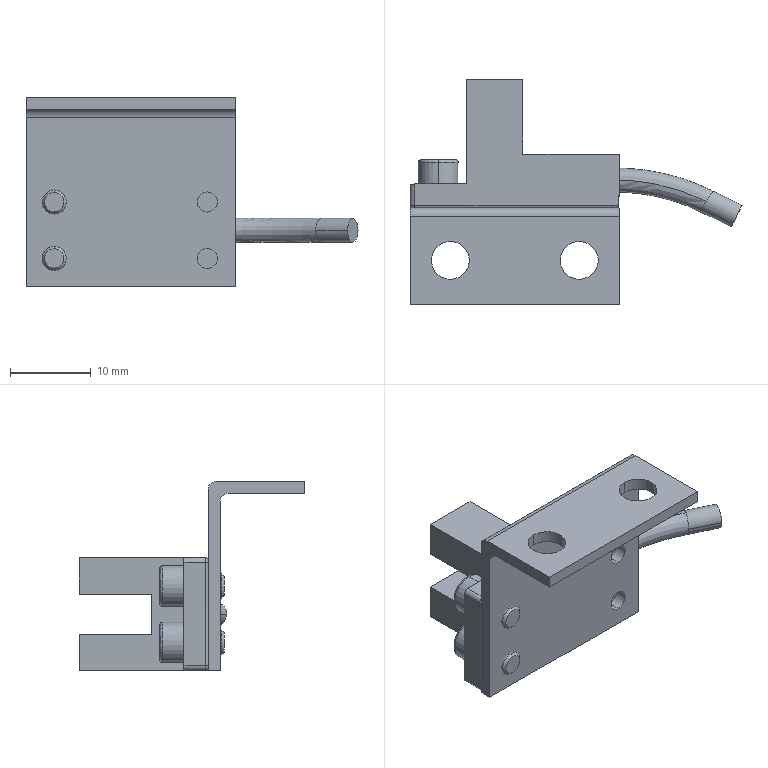Part | NX | features BREP 4 | 4 solids | 96 faces | box 41.206 x 28 x 23.5 mm | volume 4143 mm3 | plane 43 | cylinder 33 | torus 8 | spline 8 | cone 4 | commonest cylinder face diameters 3 x10 2.5 x8 4.7 x4 5 x4 0.6 x3 1.2 x2